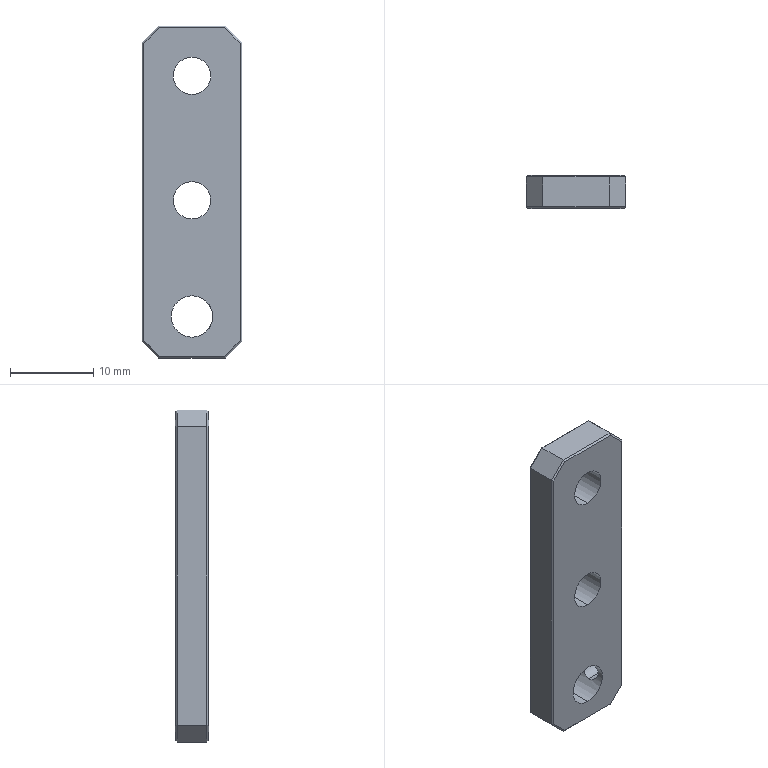Part | SolidWorks | features HoleWzd 3, Chamfer 2, Extrusion 1 | 1 solid | 34 faces | box 12 x 4 x 40 mm | volume 1661 mm3 | plane 26 | cylinder 8 | commonest cylinder face diameters 4.5 x4 2.5 x2 5 x2
STEP:
#1=CARTESIAN_POINT('',(2.165,0.,-13.75));
#2=VERTEX_POINT('',#1);
#3=CARTESIAN_POINT('',(2.165,0.,-16.25));
#4=VERTEX_POINT('',#3);
#5=CARTESIAN_POINT('',(2.165,0.,-13.75));
#6=CARTESIAN_POINT('',(2.165,-0.08275,-13.75));
#7=CARTESIAN_POINT('',(2.17,-0.1671,-13.758));
#8=CARTESIAN_POINT('',(2.188,-0.329,-13.791));
#9=CARTESIAN_POINT('',(2.202,-0.4073,-13.815));
#10=CARTESIAN_POINT('',(2.251,-0.6351,-13.911));
#11=CARTESIAN_POINT('',(2.296,-0.7703,-14.003));
#12=CARTESIAN_POINT('',(2.381,-0.9974,-14.23));
#13=CARTESIAN_POINT('',(2.423,-1.09,-14.366));
#14=CARTESIAN_POINT('',(2.482,-1.216,-14.666));
#15=CARTESIAN_POINT('',(2.5,-1.25,-14.833));
#16=CARTESIAN_POINT('',(2.5,-1.25,-15.164));
#17=CARTESIAN_POINT('',(2.483,-1.216,-15.331));
#18=CARTESIAN_POINT('',(2.423,-1.09,-15.634));
#19=CARTESIAN_POINT('',(2.381,-0.9975,-15.77));
#20=CARTESIAN_POINT('',(2.317,-0.8261,-15.942));
#21=CARTESIAN_POINT('',(2.295,-0.7643,-15.992));
#22=CARTESIAN_POINT('',(2.254,-0.6307,-16.082));
#23=CARTESIAN_POINT('',(2.235,-0.5582,-16.121));
#24=CARTESIAN_POINT('',(2.202,-0.4082,-16.184));
#25=CARTESIAN_POINT('',(2.189,-0.3303,-16.208));
#26=CARTESIAN_POINT('',(2.17,-0.1684,-16.241));
#27=CARTESIAN_POINT('',(2.165,-0.08401,-16.25));
#28=CARTESIAN_POINT('',(2.165,0.,-16.25));
#29=B_SPLINE_CURVE_WITH_KNOTS('',3,(#5,#6,#7,#8,#9,#10,#11,#12,#13,#14,#15,#16,#17,#18,#19,#20,#21,#22,#23,#24,#25,#26,#27,#28),.UNSPECIFIED.,.F.,.F.,(4,2,2,2,2,2,2,2,2,2,2,4),(0.003976,0.004224,0.004472,0.004968,0.005464,0.00596,0.006456,0.006952,0.0072,0.007448,0.007696,0.007944),.UNSPECIFIED.);
#30=EDGE_CURVE('',#2,#4,#29,.T.);
#31=ORIENTED_EDGE('',*,*,#30,.F.);
#32=CARTESIAN_POINT('',(6.,0.,-13.75));
#33=VERTEX_POINT('',#32);
#34=CARTESIAN_POINT('',(6.,0.,-13.75));
#35=DIRECTION('',(1.,0.,0.));
#36=VECTOR('',#35,1000.);
#37=LINE('',#34,#36);
#38=EDGE_CURVE('',#2,#33,#37,.T.);
#39=ORIENTED_EDGE('',*,*,#38,.T.);
#40=CARTESIAN_POINT('',(6.,0.,-16.25));
#41=VERTEX_POINT('',#40);
#42=CARTESIAN_POINT('',(6.,0.,-15.));
#43=DIRECTION('',(1.,0.,0.));
#44=DIRECTION('',(0.,0.,-1.));
#45=AXIS2_PLACEMENT_3D('',#42,#43,#44);
#46=CIRCLE('',#45,1.25);
#47=EDGE_CURVE('',#33,#41,#46,.T.);
#48=ORIENTED_EDGE('',*,*,#47,.T.);
#49=CARTESIAN_POINT('',(6.,0.,-16.25));
#50=DIRECTION('',(1.,0.,0.));
#51=VECTOR('',#50,1000.);
#52=LINE('',#49,#51);
#53=EDGE_CURVE('',#4,#41,#52,.T.);
#54=ORIENTED_EDGE('',*,*,#53,.F.);
#55=EDGE_LOOP('',(#31,#39,#48,#54));
#56=FACE_OUTER_BOUND('',#55,.T.);
#57=CARTESIAN_POINT('',(6.,0.,-15.));
#58=DIRECTION('',(1.,0.,0.));
#59=DIRECTION('',(0.,0.,-1.));
#60=AXIS2_PLACEMENT_3D('',#57,#58,#59);
#61=CYLINDRICAL_SURFACE('',#60,1.25);
#62=ADVANCED_FACE('',(#56),#61,.F.);
#63=CARTESIAN_POINT('',(0.,-2.,-3.25));
#64=VERTEX_POINT('',#63);
#65=CARTESIAN_POINT('',(0.,-2.,1.25));
#66=VERTEX_POINT('',#65);
#67=CARTESIAN_POINT('',(0.,-2.,-1.));
#68=DIRECTION('',(0.,1.,0.));
#69=DIRECTION('',(0.,0.,1.));
#70=AXIS2_PLACEMENT_3D('',#67,#68,#69);
#71=CIRCLE('',#70,2.25);
#72=EDGE_CURVE('',#64,#66,#71,.T.);
#73=ORIENTED_EDGE('',*,*,#72,.F.);
#74=CARTESIAN_POINT('',(0.,2.,-3.25));
#75=VERTEX_POINT('',#74);
#76=CARTESIAN_POINT('',(0.,2.,-3.25));
#77=DIRECTION('',(0.,1.,0.));
#78=VECTOR('',#77,1000.);
#79=LINE('',#76,#78);
#80=EDGE_CURVE('',#64,#75,#79,.T.);
#81=ORIENTED_EDGE('',*,*,#80,.T.);
#82=CARTESIAN_POINT('',(0.,2.,1.25));
#83=VERTEX_POINT('',#82);
#84=CARTESIAN_POINT('',(0.,2.,-1.));
#85=DIRECTION('',(0.,1.,0.));
#86=DIRECTION('',(0.,0.,1.));
#87=AXIS2_PLACEMENT_3D('',#84,#85,#86);
#88=CIRCLE('',#87,2.25);
#89=EDGE_CURVE('',#75,#83,#88,.T.);
#90=ORIENTED_EDGE('',*,*,#89,.T.);
#91=CARTESIAN_POINT('',(0.,2.,1.25));
#92=DIRECTION('',(0.,1.,0.));
#93=VECTOR('',#92,1000.);
#94=LINE('',#91,#93);
#95=EDGE_CURVE('',#66,#83,#94,.T.);
#96=ORIENTED_EDGE('',*,*,#95,.F.);
#97=EDGE_LOOP('',(#73,#81,#90,#96));
#98=FACE_OUTER_BOUND('',#97,.T.);
#99=CARTESIAN_POINT('',(0.,2.,-1.));
#100=DIRECTION('',(0.,1.,0.));
#101=DIRECTION('',(0.,0.,1.));
#102=AXIS2_PLACEMENT_3D('',#99,#100,#101);
#103=CYLINDRICAL_SURFACE('',#102,2.25);
#104=ADVANCED_FACE('',(#98),#103,.F.);
#105=CARTESIAN_POINT('',(0.,-2.,11.75));
#106=VERTEX_POINT('',#105);
#107=CARTESIAN_POINT('',(0.,-2.,16.25));
#108=VERTEX_POINT('',#107);
#109=CARTESIAN_POINT('',(0.,-2.,14.));
#110=DIRECTION('',(0.,1.,0.));
#111=DIRECTION('',(0.,0.,1.));
#112=AXIS2_PLACEMENT_3D('',#109,#110,#111);
#113=CIRCLE('',#112,2.25);
#114=EDGE_CURVE('',#106,#108,#113,.T.);
#115=ORIENTED_EDGE('',*,*,#114,.F.);
#116=CARTESIAN_POINT('',(0.,2.,11.75));
#117=VERTEX_POINT('',#116);
#118=CARTESIAN_POINT('',(0.,2.,11.75));
#119=DIRECTION('',(0.,1.,0.));
#120=VECTOR('',#119,1000.);
#121=LINE('',#118,#120);
#122=EDGE_CURVE('',#106,#117,#121,.T.);
#123=ORIENTED_EDGE('',*,*,#122,.T.);
#124=CARTESIAN_POINT('',(0.,2.,16.25));
#125=VERTEX_POINT('',#124);
#126=CARTESIAN_POINT('',(0.,2.,14.));
#127=DIRECTION('',(0.,1.,0.));
#128=DIRECTION('',(0.,0.,1.));
#129=AXIS2_PLACEMENT_3D('',#126,#127,#128);
#130=CIRCLE('',#129,2.25);
#131=EDGE_CURVE('',#117,#125,#130,.T.);
#132=ORIENTED_EDGE('',*,*,#131,.T.);
#133=CARTESIAN_POINT('',(0.,2.,16.25));
#134=DIRECTION('',(0.,1.,0.));
#135=VECTOR('',#134,1000.);
#136=LINE('',#133,#135);
#137=EDGE_CURVE('',#108,#125,#136,.T.);
#138=ORIENTED_EDGE('',*,*,#137,.F.);
#139=EDGE_LOOP('',(#115,#123,#132,#138));
#140=FACE_OUTER_BOUND('',#139,.T.);
#141=CARTESIAN_POINT('',(0.,2.,14.));
#142=DIRECTION('',(0.,1.,0.));
#143=DIRECTION('',(0.,0.,1.));
#144=AXIS2_PLACEMENT_3D('',#141,#142,#143);
#145=CYLINDRICAL_SURFACE('',#144,2.25);
#146=ADVANCED_FACE('',(#140),#145,.F.);
#147=CARTESIAN_POINT('',(0.,-2.,-17.5));
#148=VERTEX_POINT('',#147);
#149=CARTESIAN_POINT('',(0.,-2.,-12.5));
#150=VERTEX_POINT('',#149);
#151=CARTESIAN_POINT('',(0.,-2.,-15.));
#152=DIRECTION('',(0.,1.,0.));
#153=DIRECTION('',(0.,0.,1.));
#154=AXIS2_PLACEMENT_3D('',#151,#152,#153);
#155=CIRCLE('',#154,2.5);
#156=EDGE_CURVE('',#148,#150,#155,.T.);
#157=ORIENTED_EDGE('',*,*,#156,.F.);
#158=CARTESIAN_POINT('',(0.,2.,-17.5));
#159=VERTEX_POINT('',#158);
#160=CARTESIAN_POINT('',(0.,2.,-17.5));
#161=DIRECTION('',(0.,1.,0.));
#162=VECTOR('',#161,1000.);
#163=LINE('',#160,#162);
#164=EDGE_CURVE('',#148,#159,#163,.T.);
#165=ORIENTED_EDGE('',*,*,#164,.T.);
#166=CARTESIAN_POINT('',(0.,2.,-12.5));
#167=VERTEX_POINT('',#166);
#168=CARTESIAN_POINT('',(0.,2.,-15.));
#169=DIRECTION('',(0.,1.,0.));
#170=DIRECTION('',(0.,0.,1.));
#171=AXIS2_PLACEMENT_3D('',#168,#169,#170);
#172=CIRCLE('',#171,2.5);
#173=EDGE_CURVE('',#159,#167,#172,.T.);
#174=ORIENTED_EDGE('',*,*,#173,.T.);
#175=CARTESIAN_POINT('',(0.,2.,-12.5));
#176=DIRECTION('',(0.,1.,0.));
#177=VECTOR('',#176,1000.);
#178=LINE('',#175,#177);
#179=EDGE_CURVE('',#150,#167,#178,.T.);
#180=ORIENTED_EDGE('',*,*,#179,.F.);
#181=EDGE_LOOP('',(#157,#165,#174,#180));
#182=FACE_OUTER_BOUND('',#181,.T.);
#183=CARTESIAN_POINT('',(0.,2.,-15.));
#184=DIRECTION('',(0.,1.,0.));
#185=DIRECTION('',(0.,0.,1.));
#186=AXIS2_PLACEMENT_3D('',#183,#184,#185);
#187=CYLINDRICAL_SURFACE('',#186,2.5);
#188=ADVANCED_FACE('',(#182),#187,.F.);
#189=CARTESIAN_POINT('',(6.,0.,-15.));
#190=DIRECTION('',(1.,0.,0.));
#191=DIRECTION('',(0.,0.,-1.));
#192=AXIS2_PLACEMENT_3D('',#189,#190,#191);
#193=CIRCLE('',#192,1.25);
#194=EDGE_CURVE('',#41,#33,#193,.T.);
#195=ORIENTED_EDGE('',*,*,#194,.F.);
#196=ORIENTED_EDGE('',*,*,#47,.F.);
#197=EDGE_LOOP('',(#195,#196));
#198=FACE_BOUND('',#197,.T.);
#199=CARTESIAN_POINT('',(6.,-1.8,-18.));
#200=VERTEX_POINT('',#199);
#201=CARTESIAN_POINT('',(6.,1.8,-18.));
#202=VERTEX_POINT('',#201);
#203=CARTESIAN_POINT('',(6.,2.,-18.));
#204=DIRECTION('',(0.,1.,0.));
#205=VECTOR('',#204,1000.);
#206=LINE('',#203,#205);
#207=EDGE_CURVE('',#200,#202,#206,.T.);
#208=ORIENTED_EDGE('',*,*,#207,.T.);
#209=CARTESIAN_POINT('',(6.,1.8,18.));
#210=VERTEX_POINT('',#209);
#211=CARTESIAN_POINT('',(6.,1.8,18.));
#212=DIRECTION('',(0.,0.,1.));
#213=VECTOR('',#212,1000.);
#214=LINE('',#211,#213);
#215=EDGE_CURVE('',#202,#210,#214,.T.);
#216=ORIENTED_EDGE('',*,*,#215,.T.);
#217=CARTESIAN_POINT('',(6.,-1.8,18.));
#218=VERTEX_POINT('',#217);
#219=CARTESIAN_POINT('',(6.,2.,18.));
#220=DIRECTION('',(0.,-1.,0.));
#221=VECTOR('',#220,1000.);
#222=LINE('',#219,#221);
#223=EDGE_CURVE('',#210,#218,#222,.T.);
#224=ORIENTED_EDGE('',*,*,#223,.T.);
#225=CARTESIAN_POINT('',(6.,-1.8,-20.));
#226=DIRECTION('',(0.,0.,-1.));
#227=VECTOR('',#226,1000.);
#228=LINE('',#225,#227);
#229=EDGE_CURVE('',#218,#200,#228,.T.);
#230=ORIENTED_EDGE('',*,*,#229,.T.);
#231=EDGE_LOOP('',(#208,#216,#224,#230));
#232=FACE_OUTER_BOUND('',#231,.T.);
#233=CARTESIAN_POINT('',(6.,2.,-20.));
#234=DIRECTION('',(-1.,0.,0.));
#235=DIRECTION('',(0.,0.,1.));
#236=AXIS2_PLACEMENT_3D('',#233,#234,#235);
#237=PLANE('',#236);
#238=ADVANCED_FACE('',(#198,#232),#237,.F.);
#239=CARTESIAN_POINT('',(-4.,-1.8,-20.));
#240=VERTEX_POINT('',#239);
#241=CARTESIAN_POINT('',(-4.,1.8,-20.));
#242=VERTEX_POINT('',#241);
#243=CARTESIAN_POINT('',(-4.,2.,-20.));
#244=DIRECTION('',(0.,1.,0.));
#245=VECTOR('',#244,1000.);
#246=LINE('',#243,#245);
#247=EDGE_CURVE('',#240,#242,#246,.T.);
#248=ORIENTED_EDGE('',*,*,#247,.T.);
#249=CARTESIAN_POINT('',(4.,1.8,-20.));
#250=VERTEX_POINT('',#249);
#251=CARTESIAN_POINT('',(4.,1.8,-20.));
#252=DIRECTION('',(1.,0.,0.));
#253=VECTOR('',#252,1000.);
#254=LINE('',#251,#253);
#255=EDGE_CURVE('',#242,#250,#254,.T.);
#256=ORIENTED_EDGE('',*,*,#255,.T.);
#257=CARTESIAN_POINT('',(4.,-1.8,-20.));
#258=VERTEX_POINT('',#257);
#259=CARTESIAN_POINT('',(4.,2.,-20.));
#260=DIRECTION('',(0.,-1.,0.));
#261=VECTOR('',#260,1000.);
#262=LINE('',#259,#261);
#263=EDGE_CURVE('',#250,#258,#262,.T.);
#264=ORIENTED_EDGE('',*,*,#263,.T.);
#265=CARTESIAN_POINT('',(-6.,-1.8,-20.));
#266=DIRECTION('',(-1.,0.,0.));
#267=VECTOR('',#266,1000.);
#268=LINE('',#265,#267);
#269=EDGE_CURVE('',#258,#240,#268,.T.);
#270=ORIENTED_EDGE('',*,*,#269,.T.);
#271=EDGE_LOOP('',(#248,#256,#264,#270));
#272=FACE_OUTER_BOUND('',#271,.T.);
#273=CARTESIAN_POINT('',(-6.,2.,-20.));
#274=DIRECTION('',(0.,0.,1.));
#275=DIRECTION('',(1.,0.,0.));
#276=AXIS2_PLACEMENT_3D('',#273,#274,#275);
#277=PLANE('',#276);
#278=ADVANCED_FACE('',(#272),#277,.F.);
#279=CARTESIAN_POINT('',(-6.,-1.8,18.));
#280=VERTEX_POINT('',#279);
#281=CARTESIAN_POINT('',(-6.,1.8,18.));
#282=VERTEX_POINT('',#281);
#283=CARTESIAN_POINT('',(-6.,2.,18.));
#284=DIRECTION('',(0.,1.,0.));
#285=VECTOR('',#284,1000.);
#286=LINE('',#283,#285);
#287=EDGE_CURVE('',#280,#282,#286,.T.);
#288=ORIENTED_EDGE('',*,*,#287,.T.);
#289=CARTESIAN_POINT('',(-6.,1.8,-18.));
#290=VERTEX_POINT('',#289);
#291=CARTESIAN_POINT('',(-6.,1.8,-18.));
#292=DIRECTION('',(0.,0.,-1.));
#293=VECTOR('',#292,1000.);
#294=LINE('',#291,#293);
#295=EDGE_CURVE('',#282,#290,#294,.T.);
#296=ORIENTED_EDGE('',*,*,#295,.T.);
#297=CARTESIAN_POINT('',(-6.,-1.8,-18.));
#298=VERTEX_POINT('',#297);
#299=CARTESIAN_POINT('',(-6.,2.,-18.));
#300=DIRECTION('',(0.,-1.,0.));
#301=VECTOR('',#300,1000.);
#302=LINE('',#299,#301);
#303=EDGE_CURVE('',#290,#298,#302,.T.);
#304=ORIENTED_EDGE('',*,*,#303,.T.);
#305=CARTESIAN_POINT('',(-6.,-1.8,-20.));
#306=DIRECTION('',(0.,0.,1.));
#307=VECTOR('',#306,1000.);
#308=LINE('',#305,#307);
#309=EDGE_CURVE('',#298,#280,#308,.T.);
#310=ORIENTED_EDGE('',*,*,#309,.T.);
#311=EDGE_LOOP('',(#288,#296,#304,#310));
#312=FACE_OUTER_BOUND('',#311,.T.);
#313=CARTESIAN_POINT('',(-6.,2.,-20.));
#314=DIRECTION('',(1.,0.,0.));
#315=DIRECTION('',(0.,0.,-1.));
#316=AXIS2_PLACEMENT_3D('',#313,#314,#315);
#317=PLANE('',#316);
#318=ADVANCED_FACE('',(#312),#317,.F.);
#319=CARTESIAN_POINT('',(4.,-1.8,20.));
#320=VERTEX_POINT('',#319);
#321=CARTESIAN_POINT('',(4.,1.8,20.));
#322=VERTEX_POINT('',#321);
#323=CARTESIAN_POINT('',(4.,2.,20.));
#324=DIRECTION('',(0.,1.,0.));
#325=VECTOR('',#324,1000.);
#326=LINE('',#323,#325);
#327=EDGE_CURVE('',#320,#322,#326,.T.);
#328=ORIENTED_EDGE('',*,*,#327,.T.);
#329=CARTESIAN_POINT('',(-4.,1.8,20.));
#330=VERTEX_POINT('',#329);
#331=CARTESIAN_POINT('',(-4.,1.8,20.));
#332=DIRECTION('',(-1.,0.,0.));
#333=VECTOR('',#332,1000.);
#334=LINE('',#331,#333);
#335=EDGE_CURVE('',#322,#330,#334,.T.);
#336=ORIENTED_EDGE('',*,*,#335,.T.);
#337=CARTESIAN_POINT('',(-4.,-1.8,20.));
#338=VERTEX_POINT('',#337);
#339=CARTESIAN_POINT('',(-4.,2.,20.));
#340=DIRECTION('',(0.,-1.,0.));
#341=VECTOR('',#340,1000.);
#342=LINE('',#339,#341);
#343=EDGE_CURVE('',#330,#338,#342,.T.);
#344=ORIENTED_EDGE('',*,*,#343,.T.);
#345=CARTESIAN_POINT('',(-6.,-1.8,20.));
#346=DIRECTION('',(1.,0.,0.));
#347=VECTOR('',#346,1000.);
#348=LINE('',#345,#347);
#349=EDGE_CURVE('',#338,#320,#348,.T.);
#350=ORIENTED_EDGE('',*,*,#349,.T.);
#351=EDGE_LOOP('',(#328,#336,#344,#350));
#352=FACE_OUTER_BOUND('',#351,.T.);
#353=CARTESIAN_POINT('',(-6.,2.,20.));
#354=DIRECTION('',(0.,0.,-1.));
#355=DIRECTION('',(-1.,0.,0.));
#356=AXIS2_PLACEMENT_3D('',#353,#354,#355);
#357=PLANE('',#356);
#358=ADVANCED_FACE('',(#352),#357,.F.);
#359=CARTESIAN_POINT('',(-5.8,2.,-17.917));
#360=VERTEX_POINT('',#359);
#361=CARTESIAN_POINT('',(-5.8,2.,17.917));
#362=VERTEX_POINT('',#361);
#363=CARTESIAN_POINT('',(-5.8,2.,18.));
#364=DIRECTION('',(0.,0.,1.));
#365=VECTOR('',#364,1000.);
#366=LINE('',#363,#365);
#367=EDGE_CURVE('',#360,#362,#366,.T.);
#368=ORIENTED_EDGE('',*,*,#367,.T.);
#369=CARTESIAN_POINT('',(-3.917,2.,19.8));
#370=VERTEX_POINT('',#369);
#371=CARTESIAN_POINT('',(-11.859,2.,11.859));
#372=DIRECTION('',(0.7071,0.,0.7071));
#373=VECTOR('',#372,1000.);
#374=LINE('',#371,#373);
#375=EDGE_CURVE('',#362,#370,#374,.T.);
#376=ORIENTED_EDGE('',*,*,#375,.T.);
#377=CARTESIAN_POINT('',(3.917,2.,19.8));
#378=VERTEX_POINT('',#377);
#379=CARTESIAN_POINT('',(4.,2.,19.8));
#380=DIRECTION('',(1.,0.,0.));
#381=VECTOR('',#380,1000.);
#382=LINE('',#379,#381);
#383=EDGE_CURVE('',#370,#378,#382,.T.);
#384=ORIENTED_EDGE('',*,*,#383,.T.);
#385=CARTESIAN_POINT('',(5.8,2.,17.917));
#386=VERTEX_POINT('',#385);
#387=CARTESIAN_POINT('',(11.859,2.,11.859));
#388=DIRECTION('',(0.7071,0.,-0.7071));
#389=VECTOR('',#388,1000.);
#390=LINE('',#387,#389);
#391=EDGE_CURVE('',#378,#386,#390,.T.);
#392=ORIENTED_EDGE('',*,*,#391,.T.);
#393=CARTESIAN_POINT('',(5.8,2.,-17.917));
#394=VERTEX_POINT('',#393);
#395=CARTESIAN_POINT('',(5.8,2.,-18.));
#396=DIRECTION('',(0.,0.,-1.));
#397=VECTOR('',#396,1000.);
#398=LINE('',#395,#397);
#399=EDGE_CURVE('',#386,#394,#398,.T.);
#400=ORIENTED_EDGE('',*,*,#399,.T.);
#401=CARTESIAN_POINT('',(3.917,2.,-19.8));
#402=VERTEX_POINT('',#401);
#403=CARTESIAN_POINT('',(11.859,2.,-11.859));
#404=DIRECTION('',(-0.7071,0.,-0.7071));
#405=VECTOR('',#404,1000.);
#406=LINE('',#403,#405);
#407=EDGE_CURVE('',#394,#402,#406,.T.);
#408=ORIENTED_EDGE('',*,*,#407,.T.);
#409=CARTESIAN_POINT('',(-3.917,2.,-19.8));
#410=VERTEX_POINT('',#409);
#411=CARTESIAN_POINT('',(-4.,2.,-19.8));
#412=DIRECTION('',(-1.,0.,0.));
#413=VECTOR('',#412,1000.);
#414=LINE('',#411,#413);
#415=EDGE_CURVE('',#402,#410,#414,.T.);
#416=ORIENTED_EDGE('',*,*,#415,.T.);
#417=CARTESIAN_POINT('',(-11.859,2.,-11.859));
#418=DIRECTION('',(-0.7071,0.,0.7071));
#419=VECTOR('',#418,1000.);
#420=LINE('',#417,#419);
#421=EDGE_CURVE('',#410,#360,#420,.T.);
#422=ORIENTED_EDGE('',*,*,#421,.T.);
#423=EDGE_LOOP('',(#368,#376,#384,#392,#400,#408,#416,#422));
#424=FACE_OUTER_BOUND('',#423,.T.);
#425=CARTESIAN_POINT('',(0.,2.,-1.));
#426=DIRECTION('',(0.,1.,0.));
#427=DIRECTION('',(0.,0.,1.));
#428=AXIS2_PLACEMENT_3D('',#425,#426,#427);
#429=CIRCLE('',#428,2.25);
#430=EDGE_CURVE('',#83,#75,#429,.T.);
#431=ORIENTED_EDGE('',*,*,#430,.F.);
#432=ORIENTED_EDGE('',*,*,#89,.F.);
#433=EDGE_LOOP('',(#431,#432));
#434=FACE_BOUND('',#433,.T.);
#435=CARTESIAN_POINT('',(0.,2.,14.));
#436=DIRECTION('',(0.,1.,0.));
#437=DIRECTION('',(0.,0.,1.));
#438=AXIS2_PLACEMENT_3D('',#435,#436,#437);
#439=CIRCLE('',#438,2.25);
#440=EDGE_CURVE('',#125,#117,#439,.T.);
#441=ORIENTED_EDGE('',*,*,#440,.F.);
#442=ORIENTED_EDGE('',*,*,#131,.F.);
#443=EDGE_LOOP('',(#441,#442));
#444=FACE_BOUND('',#443,.T.);
#445=CARTESIAN_POINT('',(0.,2.,-15.));
#446=DIRECTION('',(0.,1.,0.));
#447=DIRECTION('',(0.,0.,1.));
#448=AXIS2_PLACEMENT_3D('',#445,#446,#447);
#449=CIRCLE('',#448,2.5);
#450=EDGE_CURVE('',#167,#159,#449,.T.);
#451=ORIENTED_EDGE('',*,*,#450,.F.);
#452=ORIENTED_EDGE('',*,*,#173,.F.);
#453=EDGE_LOOP('',(#451,#452));
#454=FACE_BOUND('',#453,.T.);
#455=CARTESIAN_POINT('',(0.,2.,0.));
#456=DIRECTION('',(0.,1.,0.));
#457=DIRECTION('',(0.,0.,1.));
#458=AXIS2_PLACEMENT_3D('',#455,#456,#457);
#459=PLANE('',#458);
#460=ADVANCED_FACE('',(#424,#434,#444,#454),#459,.T.);
#461=CARTESIAN_POINT('',(3.917,-2.,19.8));
#462=VERTEX_POINT('',#461);
#463=CARTESIAN_POINT('',(-3.917,-2.,19.8));
#464=VERTEX_POINT('',#463);
#465=CARTESIAN_POINT('',(0.,-2.,19.8));
#466=DIRECTION('',(-1.,0.,0.));
#467=VECTOR('',#466,1000.);
#468=LINE('',#465,#467);
#469=EDGE_CURVE('',#462,#464,#468,.T.);
#470=ORIENTED_EDGE('',*,*,#469,.T.);
#471=CARTESIAN_POINT('',(-5.8,-2.,17.917));
#472=VERTEX_POINT('',#471);
#473=CARTESIAN_POINT('',(-5.859,-2.,17.859));
#474=DIRECTION('',(-0.7071,0.,-0.7071));
#475=VECTOR('',#474,1000.);
#476=LINE('',#473,#475);
#477=EDGE_CURVE('',#464,#472,#476,.T.);
#478=ORIENTED_EDGE('',*,*,#477,.T.);
#479=CARTESIAN_POINT('',(-5.8,-2.,-17.917));
#480=VERTEX_POINT('',#479);
#481=CARTESIAN_POINT('',(-5.8,-2.,0.));
#482=DIRECTION('',(0.,0.,-1.));
#483=VECTOR('',#482,1000.);
#484=LINE('',#481,#483);
#485=EDGE_CURVE('',#472,#480,#484,.T.);
#486=ORIENTED_EDGE('',*,*,#485,.T.);
#487=CARTESIAN_POINT('',(-3.917,-2.,-19.8));
#488=VERTEX_POINT('',#487);
#489=CARTESIAN_POINT('',(-3.859,-2.,-19.859));
#490=DIRECTION('',(0.7071,0.,-0.7071));
#491=VECTOR('',#490,1000.);
#492=LINE('',#489,#491);
#493=EDGE_CURVE('',#480,#488,#492,.T.);
#494=ORIENTED_EDGE('',*,*,#493,.T.);
#495=CARTESIAN_POINT('',(3.917,-2.,-19.8));
#496=VERTEX_POINT('',#495);
#497=CARTESIAN_POINT('',(0.,-2.,-19.8));
#498=DIRECTION('',(1.,0.,0.));
#499=VECTOR('',#498,1000.);
#500=LINE('',#497,#499);
#501=EDGE_CURVE('',#488,#496,#500,.T.);
#502=ORIENTED_EDGE('',*,*,#501,.T.);
#503=CARTESIAN_POINT('',(5.8,-2.,-17.917));
#504=VERTEX_POINT('',#503);
#505=CARTESIAN_POINT('',(5.859,-2.,-17.859));
#506=DIRECTION('',(0.7071,0.,0.7071));
#507=VECTOR('',#506,1000.);
#508=LINE('',#505,#507);
#509=EDGE_CURVE('',#496,#504,#508,.T.);
#510=ORIENTED_EDGE('',*,*,#509,.T.);
#511=CARTESIAN_POINT('',(5.8,-2.,17.917));
#512=VERTEX_POINT('',#511);
#513=CARTESIAN_POINT('',(5.8,-2.,0.));
#514=DIRECTION('',(0.,0.,1.));
#515=VECTOR('',#514,1000.);
#516=LINE('',#513,#515);
#517=EDGE_CURVE('',#504,#512,#516,.T.);
#518=ORIENTED_EDGE('',*,*,#517,.T.);
#519=CARTESIAN_POINT('',(3.859,-2.,19.859));
#520=DIRECTION('',(-0.7071,0.,0.7071));
#521=VECTOR('',#520,1000.);
#522=LINE('',#519,#521);
#523=EDGE_CURVE('',#512,#462,#522,.T.);
#524=ORIENTED_EDGE('',*,*,#523,.T.);
#525=EDGE_LOOP('',(#470,#478,#486,#494,#502,#510,#518,#524));
#526=FACE_OUTER_BOUND('',#525,.T.);
#527=CARTESIAN_POINT('',(0.,-2.,-1.));
#528=DIRECTION('',(0.,1.,0.));
#529=DIRECTION('',(0.,0.,1.));
#530=AXIS2_PLACEMENT_3D('',#527,#528,#529);
#531=CIRCLE('',#530,2.25);
#532=EDGE_CURVE('',#66,#64,#531,.T.);
#533=ORIENTED_EDGE('',*,*,#532,.T.);
#534=ORIENTED_EDGE('',*,*,#72,.T.);
#535=EDGE_LOOP('',(#533,#534));
#536=FACE_BOUND('',#535,.T.);
#537=CARTESIAN_POINT('',(0.,-2.,14.));
#538=DIRECTION('',(0.,1.,0.));
#539=DIRECTION('',(0.,0.,1.));
#540=AXIS2_PLACEMENT_3D('',#537,#538,#539);
#541=CIRCLE('',#540,2.25);
#542=EDGE_CURVE('',#108,#106,#541,.T.);
#543=ORIENTED_EDGE('',*,*,#542,.T.);
#544=ORIENTED_EDGE('',*,*,#114,.T.);
#545=EDGE_LOOP('',(#543,#544));
#546=FACE_BOUND('',#545,.T.);
#547=CARTESIAN_POINT('',(0.,-2.,-15.));
#548=DIRECTION('',(0.,1.,0.));
#549=DIRECTION('',(0.,0.,1.));
#550=AXIS2_PLACEMENT_3D('',#547,#548,#549);
#551=CIRCLE('',#550,2.5);
#552=EDGE_CURVE('',#150,#148,#551,.T.);
#553=ORIENTED_EDGE('',*,*,#552,.T.);
#554=ORIENTED_EDGE('',*,*,#156,.T.);
#555=EDGE_LOOP('',(#553,#554));
#556=FACE_BOUND('',#555,.T.);
#557=CARTESIAN_POINT('',(0.,-2.,0.));
#558=DIRECTION('',(0.,1.,0.));
#559=DIRECTION('',(0.,0.,1.));
#560=AXIS2_PLACEMENT_3D('',#557,#558,#559);
#561=PLANE('',#560);
#562=ADVANCED_FACE('',(#526,#536,#546,#556),#561,.F.);
#563=ORIENTED_EDGE('',*,*,#303,.F.);
#564=CARTESIAN_POINT('',(-6.,1.8,-18.));
#565=DIRECTION('',(0.7071,0.,-0.7071));
#566=VECTOR('',#565,1000.);
#567=LINE('',#564,#566);
#568=EDGE_CURVE('',#290,#242,#567,.T.);
#569=ORIENTED_EDGE('',*,*,#568,.T.);
#570=ORIENTED_EDGE('',*,*,#247,.F.);
#571=CARTESIAN_POINT('',(-6.,-1.8,-18.));
#572=DIRECTION('',(-0.7071,0.,0.7071));
#573=VECTOR('',#572,1000.);
#574=LINE('',#571,#573);
#575=EDGE_CURVE('',#240,#298,#574,.T.);
#576=ORIENTED_EDGE('',*,*,#575,.T.);
#577=EDGE_LOOP('',(#563,#569,#570,#576));
#578=FACE_OUTER_BOUND('',#577,.T.);
#579=CARTESIAN_POINT('',(-6.,2.,-18.));
#580=DIRECTION('',(0.7071,0.,0.7071));
#581=DIRECTION('',(0.,-1.,0.));
#582=AXIS2_PLACEMENT_3D('',#579,#580,#581);
#583=PLANE('',#582);
#584=ADVANCED_FACE('',(#578),#583,.F.);
#585=ORIENTED_EDGE('',*,*,#263,.F.);
#586=CARTESIAN_POINT('',(4.,1.8,-20.));
#587=DIRECTION('',(0.7071,0.,0.7071));
#588=VECTOR('',#587,1000.);
#589=LINE('',#586,#588);
#590=EDGE_CURVE('',#250,#202,#589,.T.);
#591=ORIENTED_EDGE('',*,*,#590,.T.);
#592=ORIENTED_EDGE('',*,*,#207,.F.);
#593=CARTESIAN_POINT('',(4.,-1.8,-20.));
#594=DIRECTION('',(-0.7071,0.,-0.7071));
#595=VECTOR('',#594,1000.);
#596=LINE('',#593,#595);
#597=EDGE_CURVE('',#200,#258,#596,.T.);
#598=ORIENTED_EDGE('',*,*,#597,.T.);
#599=EDGE_LOOP('',(#585,#591,#592,#598));
#600=FACE_OUTER_BOUND('',#599,.T.);
#601=CARTESIAN_POINT('',(4.,2.,-20.));
#602=DIRECTION('',(-0.7071,0.,0.7071));
#603=DIRECTION('',(0.,-1.,0.));
#604=AXIS2_PLACEMENT_3D('',#601,#602,#603);
#605=PLANE('',#604);
#606=ADVANCED_FACE('',(#600),#605,.F.);
#607=ORIENTED_EDGE('',*,*,#223,.F.);
#608=CARTESIAN_POINT('',(6.,1.8,18.));
#609=DIRECTION('',(-0.7071,0.,0.7071));
#610=VECTOR('',#609,1000.);
#611=LINE('',#608,#610);
#612=EDGE_CURVE('',#210,#322,#611,.T.);
#613=ORIENTED_EDGE('',*,*,#612,.T.);
#614=ORIENTED_EDGE('',*,*,#327,.F.);
#615=CARTESIAN_POINT('',(6.,-1.8,18.));
#616=DIRECTION('',(0.7071,0.,-0.7071));
#617=VECTOR('',#616,1000.);
#618=LINE('',#615,#617);
#619=EDGE_CURVE('',#320,#218,#618,.T.);
#620=ORIENTED_EDGE('',*,*,#619,.T.);
#621=EDGE_LOOP('',(#607,#613,#614,#620));
#622=FACE_OUTER_BOUND('',#621,.T.);
#623=CARTESIAN_POINT('',(6.,2.,18.));
#624=DIRECTION('',(-0.7071,0.,-0.7071));
#625=DIRECTION('',(0.,-1.,0.));
#626=AXIS2_PLACEMENT_3D('',#623,#624,#625);
#627=PLANE('',#626);
#628=ADVANCED_FACE('',(#622),#627,.F.);
#629=ORIENTED_EDGE('',*,*,#343,.F.);
#630=CARTESIAN_POINT('',(-4.,1.8,20.));
#631=DIRECTION('',(-0.7071,0.,-0.7071));
#632=VECTOR('',#631,1000.);
#633=LINE('',#630,#632);
#634=EDGE_CURVE('',#330,#282,#633,.T.);
#635=ORIENTED_EDGE('',*,*,#634,.T.);
#636=ORIENTED_EDGE('',*,*,#287,.F.);
#637=CARTESIAN_POINT('',(-4.,-1.8,20.));
#638=DIRECTION('',(0.7071,0.,0.7071));
#639=VECTOR('',#638,1000.);
#640=LINE('',#637,#639);
#641=EDGE_CURVE('',#280,#338,#640,.T.);
#642=ORIENTED_EDGE('',*,*,#641,.T.);
#643=EDGE_LOOP('',(#629,#635,#636,#642));
#644=FACE_OUTER_BOUND('',#643,.T.);
#645=CARTESIAN_POINT('',(-4.,2.,20.));
#646=DIRECTION('',(0.7071,0.,-0.7071));
#647=DIRECTION('',(0.,-1.,0.));
#648=AXIS2_PLACEMENT_3D('',#645,#646,#647);
#649=PLANE('',#648);
#650=ADVANCED_FACE('',(#644),#649,.F.);
#651=ORIENTED_EDGE('',*,*,#164,.F.);
#652=ORIENTED_EDGE('',*,*,#552,.F.);
#653=ORIENTED_EDGE('',*,*,#179,.T.);
#654=ORIENTED_EDGE('',*,*,#450,.T.);
#655=EDGE_LOOP('',(#651,#652,#653,#654));
#656=FACE_OUTER_BOUND('',#655,.T.);
#657=CARTESIAN_POINT('',(2.165,0.,-16.25));
#658=CARTESIAN_POINT('',(2.165,0.08416,-16.25));
#659=CARTESIAN_POINT('',(2.17,0.1666,-16.242));
#660=CARTESIAN_POINT('',(2.188,0.3281,-16.209));
#661=CARTESIAN_POINT('',(2.202,0.4081,-16.184));
#662=CARTESIAN_POINT('',(2.251,0.6338,-16.09));
#663=CARTESIAN_POINT('',(2.296,0.7701,-15.998));
#664=CARTESIAN_POINT('',(2.381,0.9969,-15.771));
#665=CARTESIAN_POINT('',(2.423,1.09,-15.634));
#666=CARTESIAN_POINT('',(2.468,1.184,-15.409));
#667=CARTESIAN_POINT('',(2.48,1.209,-15.329));
#668=CARTESIAN_POINT('',(2.496,1.242,-15.166));
#669=CARTESIAN_POINT('',(2.5,1.25,-15.084));
#670=CARTESIAN_POINT('',(2.5,1.25,-14.834));
#671=CARTESIAN_POINT('',(2.483,1.216,-14.668));
#672=CARTESIAN_POINT('',(2.423,1.089,-14.364));
#673=CARTESIAN_POINT('',(2.381,0.9961,-14.228));
#674=CARTESIAN_POINT('',(2.295,0.7688,-14.001));
#675=CARTESIAN_POINT('',(2.251,0.6319,-13.909));
#676=CARTESIAN_POINT('',(2.186,0.3327,-13.784));
#677=CARTESIAN_POINT('',(2.165,0.1658,-13.75));
#678=CARTESIAN_POINT('',(2.165,0.,-13.75));
#679=B_SPLINE_CURVE_WITH_KNOTS('',3,(#657,#658,#659,#660,#661,#662,#663,#664,#665,#666,#667,#668,#669,#670,#671,#672,#673,#674,#675,#676,#677,#678),.UNSPECIFIED.,.F.,.F.,(4,2,2,2,2,2,2,2,2,2,4),(0.,0.0002485,0.000497,0.0009939,0.001491,0.001739,0.001988,0.002485,0.002982,0.003479,0.003976),.UNSPECIFIED.);
#680=EDGE_CURVE('',#4,#2,#679,.T.);
#681=ORIENTED_EDGE('',*,*,#680,.T.);
#682=ORIENTED_EDGE('',*,*,#30,.T.);
#683=EDGE_LOOP('',(#681,#682));
#684=FACE_BOUND('',#683,.T.);
#685=CARTESIAN_POINT('',(0.,2.,-15.));
#686=DIRECTION('',(0.,1.,0.));
#687=DIRECTION('',(0.,0.,1.));
#688=AXIS2_PLACEMENT_3D('',#685,#686,#687);
#689=CYLINDRICAL_SURFACE('',#688,2.5);
#690=ADVANCED_FACE('',(#656,#684),#689,.F.);
#691=ORIENTED_EDGE('',*,*,#122,.F.);
#692=ORIENTED_EDGE('',*,*,#542,.F.);
#693=ORIENTED_EDGE('',*,*,#137,.T.);
#694=ORIENTED_EDGE('',*,*,#440,.T.);
#695=EDGE_LOOP('',(#691,#692,#693,#694));
#696=FACE_OUTER_BOUND('',#695,.T.);
#697=CARTESIAN_POINT('',(0.,2.,14.));
#698=DIRECTION('',(0.,1.,0.));
#699=DIRECTION('',(0.,0.,1.));
#700=AXIS2_PLACEMENT_3D('',#697,#698,#699);
#701=CYLINDRICAL_SURFACE('',#700,2.25);
#702=ADVANCED_FACE('',(#696),#701,.F.);
#703=ORIENTED_EDGE('',*,*,#80,.F.);
#704=ORIENTED_EDGE('',*,*,#532,.F.);
#705=ORIENTED_EDGE('',*,*,#95,.T.);
#706=ORIENTED_EDGE('',*,*,#430,.T.);
#707=EDGE_LOOP('',(#703,#704,#705,#706));
#708=FACE_OUTER_BOUND('',#707,.T.);
#709=CARTESIAN_POINT('',(0.,2.,-1.));
#710=DIRECTION('',(0.,1.,0.));
#711=DIRECTION('',(0.,0.,1.));
#712=AXIS2_PLACEMENT_3D('',#709,#710,#711);
#713=CYLINDRICAL_SURFACE('',#712,2.25);
#714=ADVANCED_FACE('',(#708),#713,.F.);
#715=ORIENTED_EDGE('',*,*,#38,.F.);
#716=ORIENTED_EDGE('',*,*,#680,.F.);
#717=ORIENTED_EDGE('',*,*,#53,.T.);
#718=ORIENTED_EDGE('',*,*,#194,.T.);
#719=EDGE_LOOP('',(#715,#716,#717,#718));
#720=FACE_OUTER_BOUND('',#719,.T.);
#721=CARTESIAN_POINT('',(6.,0.,-15.));
#722=DIRECTION('',(1.,0.,0.));
#723=DIRECTION('',(0.,0.,-1.));
#724=AXIS2_PLACEMENT_3D('',#721,#722,#723);
#725=CYLINDRICAL_SURFACE('',#724,1.25);
#726=ADVANCED_FACE('',(#720),#725,.F.);
#727=CARTESIAN_POINT('',(2.382,5.418,-16.502));
#728=DIRECTION('',(-0.6786,0.6786,0.2811));
#729=VECTOR('',#728,1000.);
#730=LINE('',#727,#729);
#731=EDGE_CURVE('',#202,#394,#730,.T.);
#732=ORIENTED_EDGE('',*,*,#731,.F.);
#733=ORIENTED_EDGE('',*,*,#590,.F.);
#734=CARTESIAN_POINT('',(3.03,4.142,-17.658));
#735=DIRECTION('',(0.2811,-0.6786,-0.6786));
#736=VECTOR('',#735,1000.);
#737=LINE('',#734,#736);
#738=EDGE_CURVE('',#402,#250,#737,.T.);
#739=ORIENTED_EDGE('',*,*,#738,.F.);
#740=ORIENTED_EDGE('',*,*,#407,.F.);
#741=EDGE_LOOP('',(#732,#733,#739,#740));
#742=FACE_OUTER_BOUND('',#741,.T.);
#743=CARTESIAN_POINT('',(11.859,2.,-11.859));
#744=DIRECTION('',(0.5,0.7071,-0.5));
#745=DIRECTION('',(0.7071,0.,0.7071));
#746=AXIS2_PLACEMENT_3D('',#743,#744,#745);
#747=PLANE('',#746);
#748=ADVANCED_FACE('',(#742),#747,.T.);
#749=ORIENTED_EDGE('',*,*,#738,.T.);
#750=ORIENTED_EDGE('',*,*,#255,.F.);
#751=CARTESIAN_POINT('',(-3.608,2.747,-19.053));
#752=DIRECTION('',(-0.2811,-0.6786,-0.6786));
#753=VECTOR('',#752,1000.);
#754=LINE('',#751,#753);
#755=EDGE_CURVE('',#410,#242,#754,.T.);
#756=ORIENTED_EDGE('',*,*,#755,.F.);
#757=ORIENTED_EDGE('',*,*,#415,.F.);
#758=EDGE_LOOP('',(#749,#750,#756,#757));
#759=FACE_OUTER_BOUND('',#758,.T.);
#760=CARTESIAN_POINT('',(0.,2.,-19.8));
#761=DIRECTION('',(0.,0.7071,-0.7071));
#762=DIRECTION('',(1.,0.,0.));
#763=AXIS2_PLACEMENT_3D('',#760,#761,#762);
#764=PLANE('',#763);
#765=ADVANCED_FACE('',(#759),#764,.T.);
#766=ORIENTED_EDGE('',*,*,#731,.T.);
#767=ORIENTED_EDGE('',*,*,#399,.F.);
#768=CARTESIAN_POINT('',(2.382,5.418,16.502));
#769=DIRECTION('',(-0.6786,0.6786,-0.2811));
#770=VECTOR('',#769,1000.);
#771=LINE('',#768,#770);
#772=EDGE_CURVE('',#210,#386,#771,.T.);
#773=ORIENTED_EDGE('',*,*,#772,.F.);
#774=ORIENTED_EDGE('',*,*,#215,.F.);
#775=EDGE_LOOP('',(#766,#767,#773,#774));
#776=FACE_OUTER_BOUND('',#775,.T.);
#777=CARTESIAN_POINT('',(5.8,2.,0.));
#778=DIRECTION('',(0.7071,0.7071,0.));
#779=DIRECTION('',(0.,0.,1.));
#780=AXIS2_PLACEMENT_3D('',#777,#778,#779);
#781=PLANE('',#780);
#782=ADVANCED_FACE('',(#776),#781,.T.);
#783=ORIENTED_EDGE('',*,*,#755,.T.);
#784=ORIENTED_EDGE('',*,*,#568,.F.);
#785=CARTESIAN_POINT('',(-7.434,0.3657,-18.594));
#786=DIRECTION('',(-0.6786,-0.6786,-0.2811));
#787=VECTOR('',#786,1000.);
#788=LINE('',#785,#787);
#789=EDGE_CURVE('',#360,#290,#788,.T.);
#790=ORIENTED_EDGE('',*,*,#789,.F.);
#791=ORIENTED_EDGE('',*,*,#421,.F.);
#792=EDGE_LOOP('',(#783,#784,#790,#791));
#793=FACE_OUTER_BOUND('',#792,.T.);
#794=CARTESIAN_POINT('',(-11.859,2.,-11.859));
#795=DIRECTION('',(-0.5,0.7071,-0.5));
#796=DIRECTION('',(0.7071,0.,-0.7071));
#797=AXIS2_PLACEMENT_3D('',#794,#795,#796);
#798=PLANE('',#797);
#799=ADVANCED_FACE('',(#793),#798,.T.);
#800=ORIENTED_EDGE('',*,*,#772,.T.);
#801=ORIENTED_EDGE('',*,*,#391,.F.);
#802=CARTESIAN_POINT('',(3.03,4.142,17.658));
#803=DIRECTION('',(-0.2811,0.6786,-0.6786));
#804=VECTOR('',#803,1000.);
#805=LINE('',#802,#804);
#806=EDGE_CURVE('',#322,#378,#805,.T.);
#807=ORIENTED_EDGE('',*,*,#806,.F.);
#808=ORIENTED_EDGE('',*,*,#612,.F.);
#809=EDGE_LOOP('',(#800,#801,#807,#808));
#810=FACE_OUTER_BOUND('',#809,.T.);
#811=CARTESIAN_POINT('',(11.859,2.,11.859));
#812=DIRECTION('',(0.5,0.7071,0.5));
#813=DIRECTION('',(-0.7071,0.,0.7071));
#814=AXIS2_PLACEMENT_3D('',#811,#812,#813);
#815=PLANE('',#814);
#816=ADVANCED_FACE('',(#810),#815,.T.);
#817=ORIENTED_EDGE('',*,*,#789,.T.);
#818=ORIENTED_EDGE('',*,*,#295,.F.);
#819=CARTESIAN_POINT('',(-2.382,5.418,16.502));
#820=DIRECTION('',(-0.6786,-0.6786,0.2811));
#821=VECTOR('',#820,1000.);
#822=LINE('',#819,#821);
#823=EDGE_CURVE('',#362,#282,#822,.T.);
#824=ORIENTED_EDGE('',*,*,#823,.F.);
#825=ORIENTED_EDGE('',*,*,#367,.F.);
#826=EDGE_LOOP('',(#817,#818,#824,#825));
#827=FACE_OUTER_BOUND('',#826,.T.);
#828=CARTESIAN_POINT('',(-5.8,2.,0.));
#829=DIRECTION('',(-0.7071,0.7071,0.));
#830=DIRECTION('',(0.,0.,-1.));
#831=AXIS2_PLACEMENT_3D('',#828,#829,#830);
#832=PLANE('',#831);
#833=ADVANCED_FACE('',(#827),#832,.T.);
#834=ORIENTED_EDGE('',*,*,#806,.T.);
#835=ORIENTED_EDGE('',*,*,#383,.F.);
#836=CARTESIAN_POINT('',(-3.608,2.747,19.053));
#837=DIRECTION('',(0.2811,0.6786,-0.6786));
#838=VECTOR('',#837,1000.);
#839=LINE('',#836,#838);
#840=EDGE_CURVE('',#330,#370,#839,.T.);
#841=ORIENTED_EDGE('',*,*,#840,.F.);
#842=ORIENTED_EDGE('',*,*,#335,.F.);
#843=EDGE_LOOP('',(#834,#835,#841,#842));
#844=FACE_OUTER_BOUND('',#843,.T.);
#845=CARTESIAN_POINT('',(0.,2.,19.8));
#846=DIRECTION('',(0.,0.7071,0.7071));
#847=DIRECTION('',(-1.,0.,0.));
#848=AXIS2_PLACEMENT_3D('',#845,#846,#847);
#849=PLANE('',#848);
#850=ADVANCED_FACE('',(#844),#849,.T.);
#851=ORIENTED_EDGE('',*,*,#823,.T.);
#852=ORIENTED_EDGE('',*,*,#634,.F.);
#853=ORIENTED_EDGE('',*,*,#840,.T.);
#854=ORIENTED_EDGE('',*,*,#375,.F.);
#855=EDGE_LOOP('',(#851,#852,#853,#854));
#856=FACE_OUTER_BOUND('',#855,.T.);
#857=CARTESIAN_POINT('',(-11.859,2.,11.859));
#858=DIRECTION('',(-0.5,0.7071,0.5));
#859=DIRECTION('',(-0.7071,0.,-0.7071));
#860=AXIS2_PLACEMENT_3D('',#857,#858,#859);
#861=PLANE('',#860);
#862=ADVANCED_FACE('',(#856),#861,.T.);
#863=CARTESIAN_POINT('',(3.03,-4.142,-17.658));
#864=DIRECTION('',(-0.2811,-0.6786,0.6786));
#865=VECTOR('',#864,1000.);
#866=LINE('',#863,#865);
#867=EDGE_CURVE('',#258,#496,#866,.T.);
#868=ORIENTED_EDGE('',*,*,#867,.F.);
#869=ORIENTED_EDGE('',*,*,#597,.F.);
#870=CARTESIAN_POINT('',(6.381,-1.419,-18.158));
#871=DIRECTION('',(0.6786,0.6786,-0.2811));
#872=VECTOR('',#871,1000.);
#873=LINE('',#870,#872);
#874=EDGE_CURVE('',#504,#200,#873,.T.);
#875=ORIENTED_EDGE('',*,*,#874,.F.);
#876=ORIENTED_EDGE('',*,*,#509,.F.);
#877=EDGE_LOOP('',(#868,#869,#875,#876));
#878=FACE_OUTER_BOUND('',#877,.T.);
#879=CARTESIAN_POINT('',(11.859,-2.,-11.859));
#880=DIRECTION('',(-0.5,0.7071,0.5));
#881=DIRECTION('',(0.7071,0.,0.7071));
#882=AXIS2_PLACEMENT_3D('',#879,#880,#881);
#883=PLANE('',#882);
#884=ADVANCED_FACE('',(#878),#883,.F.);
#885=ORIENTED_EDGE('',*,*,#874,.T.);
#886=ORIENTED_EDGE('',*,*,#229,.F.);
#887=CARTESIAN_POINT('',(-1.248,-9.048,14.998));
#888=DIRECTION('',(0.6786,0.6786,0.2811));
#889=VECTOR('',#888,1000.);
#890=LINE('',#887,#889);
#891=EDGE_CURVE('',#512,#218,#890,.T.);
#892=ORIENTED_EDGE('',*,*,#891,.F.);
#893=ORIENTED_EDGE('',*,*,#517,.F.);
#894=EDGE_LOOP('',(#885,#886,#892,#893));
#895=FACE_OUTER_BOUND('',#894,.T.);
#896=CARTESIAN_POINT('',(6.,-1.8,-20.));
#897=DIRECTION('',(-0.7071,0.7071,0.));
#898=DIRECTION('',(0.,0.,-1.));
#899=AXIS2_PLACEMENT_3D('',#896,#897,#898);
#900=PLANE('',#899);
#901=ADVANCED_FACE('',(#895),#900,.F.);
#902=ORIENTED_EDGE('',*,*,#867,.T.);
#903=ORIENTED_EDGE('',*,*,#501,.F.);
#904=CARTESIAN_POINT('',(-4.158,-1.419,-20.381));
#905=DIRECTION('',(0.2811,-0.6786,0.6786));
#906=VECTOR('',#905,1000.);
#907=LINE('',#904,#906);
#908=EDGE_CURVE('',#240,#488,#907,.T.);
#909=ORIENTED_EDGE('',*,*,#908,.F.);
#910=ORIENTED_EDGE('',*,*,#269,.F.);
#911=EDGE_LOOP('',(#902,#903,#909,#910));
#912=FACE_OUTER_BOUND('',#911,.T.);
#913=CARTESIAN_POINT('',(-6.,-1.8,-20.));
#914=DIRECTION('',(0.,0.7071,0.7071));
#915=DIRECTION('',(-1.,0.,0.));
#916=AXIS2_PLACEMENT_3D('',#913,#914,#915);
#917=PLANE('',#916);
#918=ADVANCED_FACE('',(#912),#917,.F.);
#919=ORIENTED_EDGE('',*,*,#891,.T.);
#920=ORIENTED_EDGE('',*,*,#619,.F.);
#921=CARTESIAN_POINT('',(3.03,-4.142,17.658));
#922=DIRECTION('',(0.2811,0.6786,0.6786));
#923=VECTOR('',#922,1000.);
#924=LINE('',#921,#923);
#925=EDGE_CURVE('',#462,#320,#924,.T.);
#926=ORIENTED_EDGE('',*,*,#925,.F.);
#927=ORIENTED_EDGE('',*,*,#523,.F.);
#928=EDGE_LOOP('',(#919,#920,#926,#927));
#929=FACE_OUTER_BOUND('',#928,.T.);
#930=CARTESIAN_POINT('',(11.859,-2.,11.859));
#931=DIRECTION('',(-0.5,0.7071,-0.5));
#932=DIRECTION('',(-0.7071,0.,0.7071));
#933=AXIS2_PLACEMENT_3D('',#930,#931,#932);
#934=PLANE('',#933);
#935=ADVANCED_FACE('',(#929),#934,.F.);
#936=ORIENTED_EDGE('',*,*,#908,.T.);
#937=ORIENTED_EDGE('',*,*,#493,.F.);
#938=CARTESIAN_POINT('',(-7.434,-0.3657,-18.594));
#939=DIRECTION('',(0.6786,-0.6786,0.2811));
#940=VECTOR('',#939,1000.);
#941=LINE('',#938,#940);
#942=EDGE_CURVE('',#298,#480,#941,.T.);
#943=ORIENTED_EDGE('',*,*,#942,.F.);
#944=ORIENTED_EDGE('',*,*,#575,.F.);
#945=EDGE_LOOP('',(#936,#937,#943,#944));
#946=FACE_OUTER_BOUND('',#945,.T.);
#947=CARTESIAN_POINT('',(-11.859,-2.,-11.859));
#948=DIRECTION('',(0.5,0.7071,0.5));
#949=DIRECTION('',(0.7071,0.,-0.7071));
#950=AXIS2_PLACEMENT_3D('',#947,#948,#949);
#951=PLANE('',#950);
#952=ADVANCED_FACE('',(#946),#951,.F.);
#953=ORIENTED_EDGE('',*,*,#925,.T.);
#954=ORIENTED_EDGE('',*,*,#349,.F.);
#955=CARTESIAN_POINT('',(-4.158,-1.419,20.381));
#956=DIRECTION('',(-0.2811,0.6786,0.6786));
#957=VECTOR('',#956,1000.);
#958=LINE('',#955,#957);
#959=EDGE_CURVE('',#464,#338,#958,.T.);
#960=ORIENTED_EDGE('',*,*,#959,.F.);
#961=ORIENTED_EDGE('',*,*,#469,.F.);
#962=EDGE_LOOP('',(#953,#954,#960,#961));
#963=FACE_OUTER_BOUND('',#962,.T.);
#964=CARTESIAN_POINT('',(-6.,-1.8,20.));
#965=DIRECTION('',(0.,0.7071,-0.7071));
#966=DIRECTION('',(1.,0.,0.));
#967=AXIS2_PLACEMENT_3D('',#964,#965,#966);
#968=PLANE('',#967);
#969=ADVANCED_FACE('',(#963),#968,.F.);
#970=ORIENTED_EDGE('',*,*,#942,.T.);
#971=ORIENTED_EDGE('',*,*,#485,.F.);
#972=CARTESIAN_POINT('',(1.248,-9.048,14.998));
#973=DIRECTION('',(0.6786,-0.6786,-0.2811));
#974=VECTOR('',#973,1000.);
#975=LINE('',#972,#974);
#976=EDGE_CURVE('',#280,#472,#975,.T.);
#977=ORIENTED_EDGE('',*,*,#976,.F.);
#978=ORIENTED_EDGE('',*,*,#309,.F.);
#979=EDGE_LOOP('',(#970,#971,#977,#978));
#980=FACE_OUTER_BOUND('',#979,.T.);
#981=CARTESIAN_POINT('',(-6.,-1.8,-20.));
#982=DIRECTION('',(0.7071,0.7071,0.));
#983=DIRECTION('',(0.,0.,1.));
#984=AXIS2_PLACEMENT_3D('',#981,#982,#983);
#985=PLANE('',#984);
#986=ADVANCED_FACE('',(#980),#985,.F.);
#987=ORIENTED_EDGE('',*,*,#959,.T.);
#988=ORIENTED_EDGE('',*,*,#641,.F.);
#989=ORIENTED_EDGE('',*,*,#976,.T.);
#990=ORIENTED_EDGE('',*,*,#477,.F.);
#991=EDGE_LOOP('',(#987,#988,#989,#990));
#992=FACE_OUTER_BOUND('',#991,.T.);
#993=CARTESIAN_POINT('',(-11.859,-2.,11.859));
#994=DIRECTION('',(0.5,0.7071,-0.5));
#995=DIRECTION('',(-0.7071,0.,-0.7071));
#996=AXIS2_PLACEMENT_3D('',#993,#994,#995);
#997=PLANE('',#996);
#998=ADVANCED_FACE('',(#992),#997,.F.);
#999=CLOSED_SHELL('',(#62,#104,#146,#188,#238,#278,#318,#358,#460,#562,#584,#606,#628,#650,#690,#702,#714,#726,#748,#765,#782,#799,#816,#833,#850,#862,#884,#901,#918,#935,#952,#969,#986,#998));
#1000=MANIFOLD_SOLID_BREP('',#999);
#1001=CARTESIAN_POINT('',(0.,0.,0.));
#1002=DIRECTION('',(0.,0.,1.));
#1003=DIRECTION('',(1.,0.,0.));
#1004=AXIS2_PLACEMENT_3D('',#1001,#1002,#1003);
#1005=(LENGTH_UNIT()NAMED_UNIT(*)SI_UNIT(.MILLI.,.METRE.));
#1006=UNCERTAINTY_MEASURE_WITH_UNIT(LENGTH_MEASURE(0.00001),#1005,'','');
#1007=(NAMED_UNIT(*)PLANE_ANGLE_UNIT()SI_UNIT($,.RADIAN.));
#1008=(NAMED_UNIT(*)SI_UNIT($,.STERADIAN.)SOLID_ANGLE_UNIT());
#1009=(GEOMETRIC_REPRESENTATION_CONTEXT(3)GLOBAL_UNCERTAINTY_ASSIGNED_CONTEXT((#1006))GLOBAL_UNIT_ASSIGNED_CONTEXT((#1005,#1007,#1008))REPRESENTATION_CONTEXT('',''));
#1010=ADVANCED_BREP_SHAPE_REPRESENTATION('',(#1000,#1004),#1009);